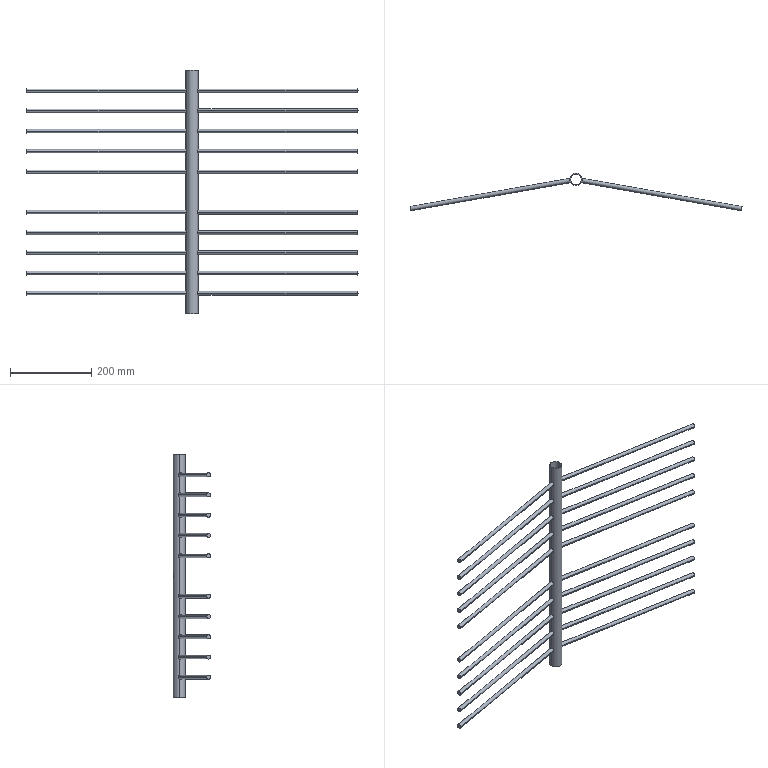Part | SolidWorks | features ICE 4, Extrusion 1 | 21 solids | 88 faces | box 819.127 x 91.988 x 600 mm | volume 708781 mm3 | cylinder 46 | plane 42 | commonest cylinder face diameters 10 x42 27 x2 30 x2